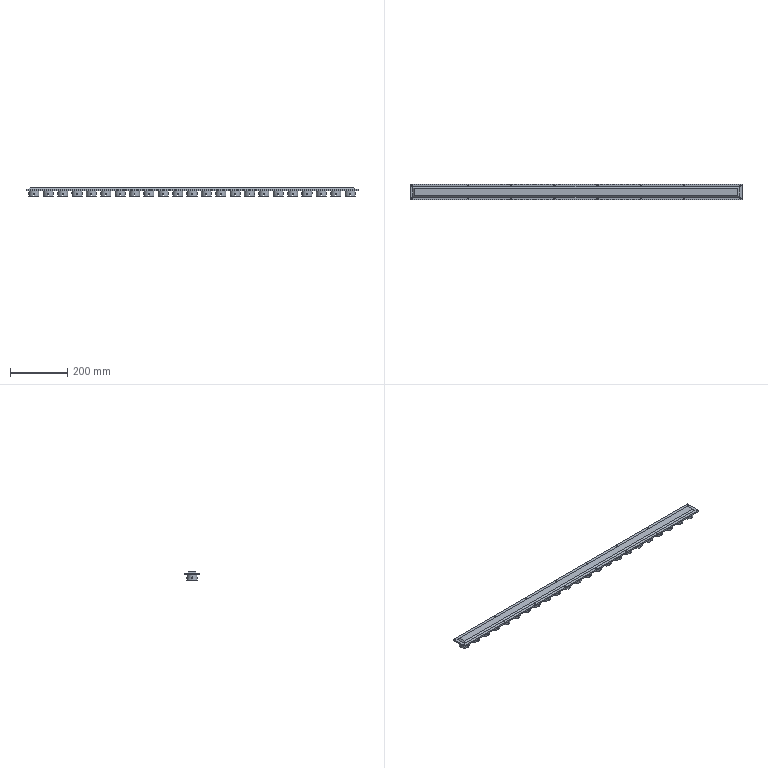Part | SolidWorks | features BaseBody 1 | 1 solid | 526 faces | box 1155 x 55 x 30 mm | volume 645147 mm3 | plane 402 | cylinder 124 | commonest cylinder face diameters 27.5 x46 35 x46 4 x32